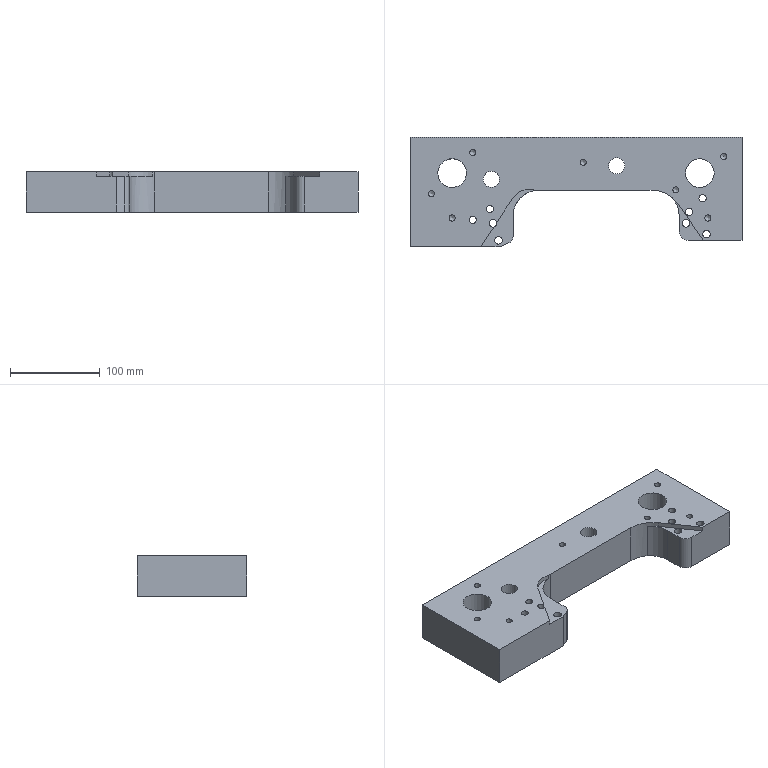Part | STEP file | 301_id2322_x_t | 1 solid | 75 faces | box 370 x 122 x 45 mm | volume 1311986 mm3 | cylinder 38 | plane 22 | cone 15 | commonest cylinder face diameters 6.8 x11 8 x4 8.5 x4 5.52 x2 10 x2 14 x2